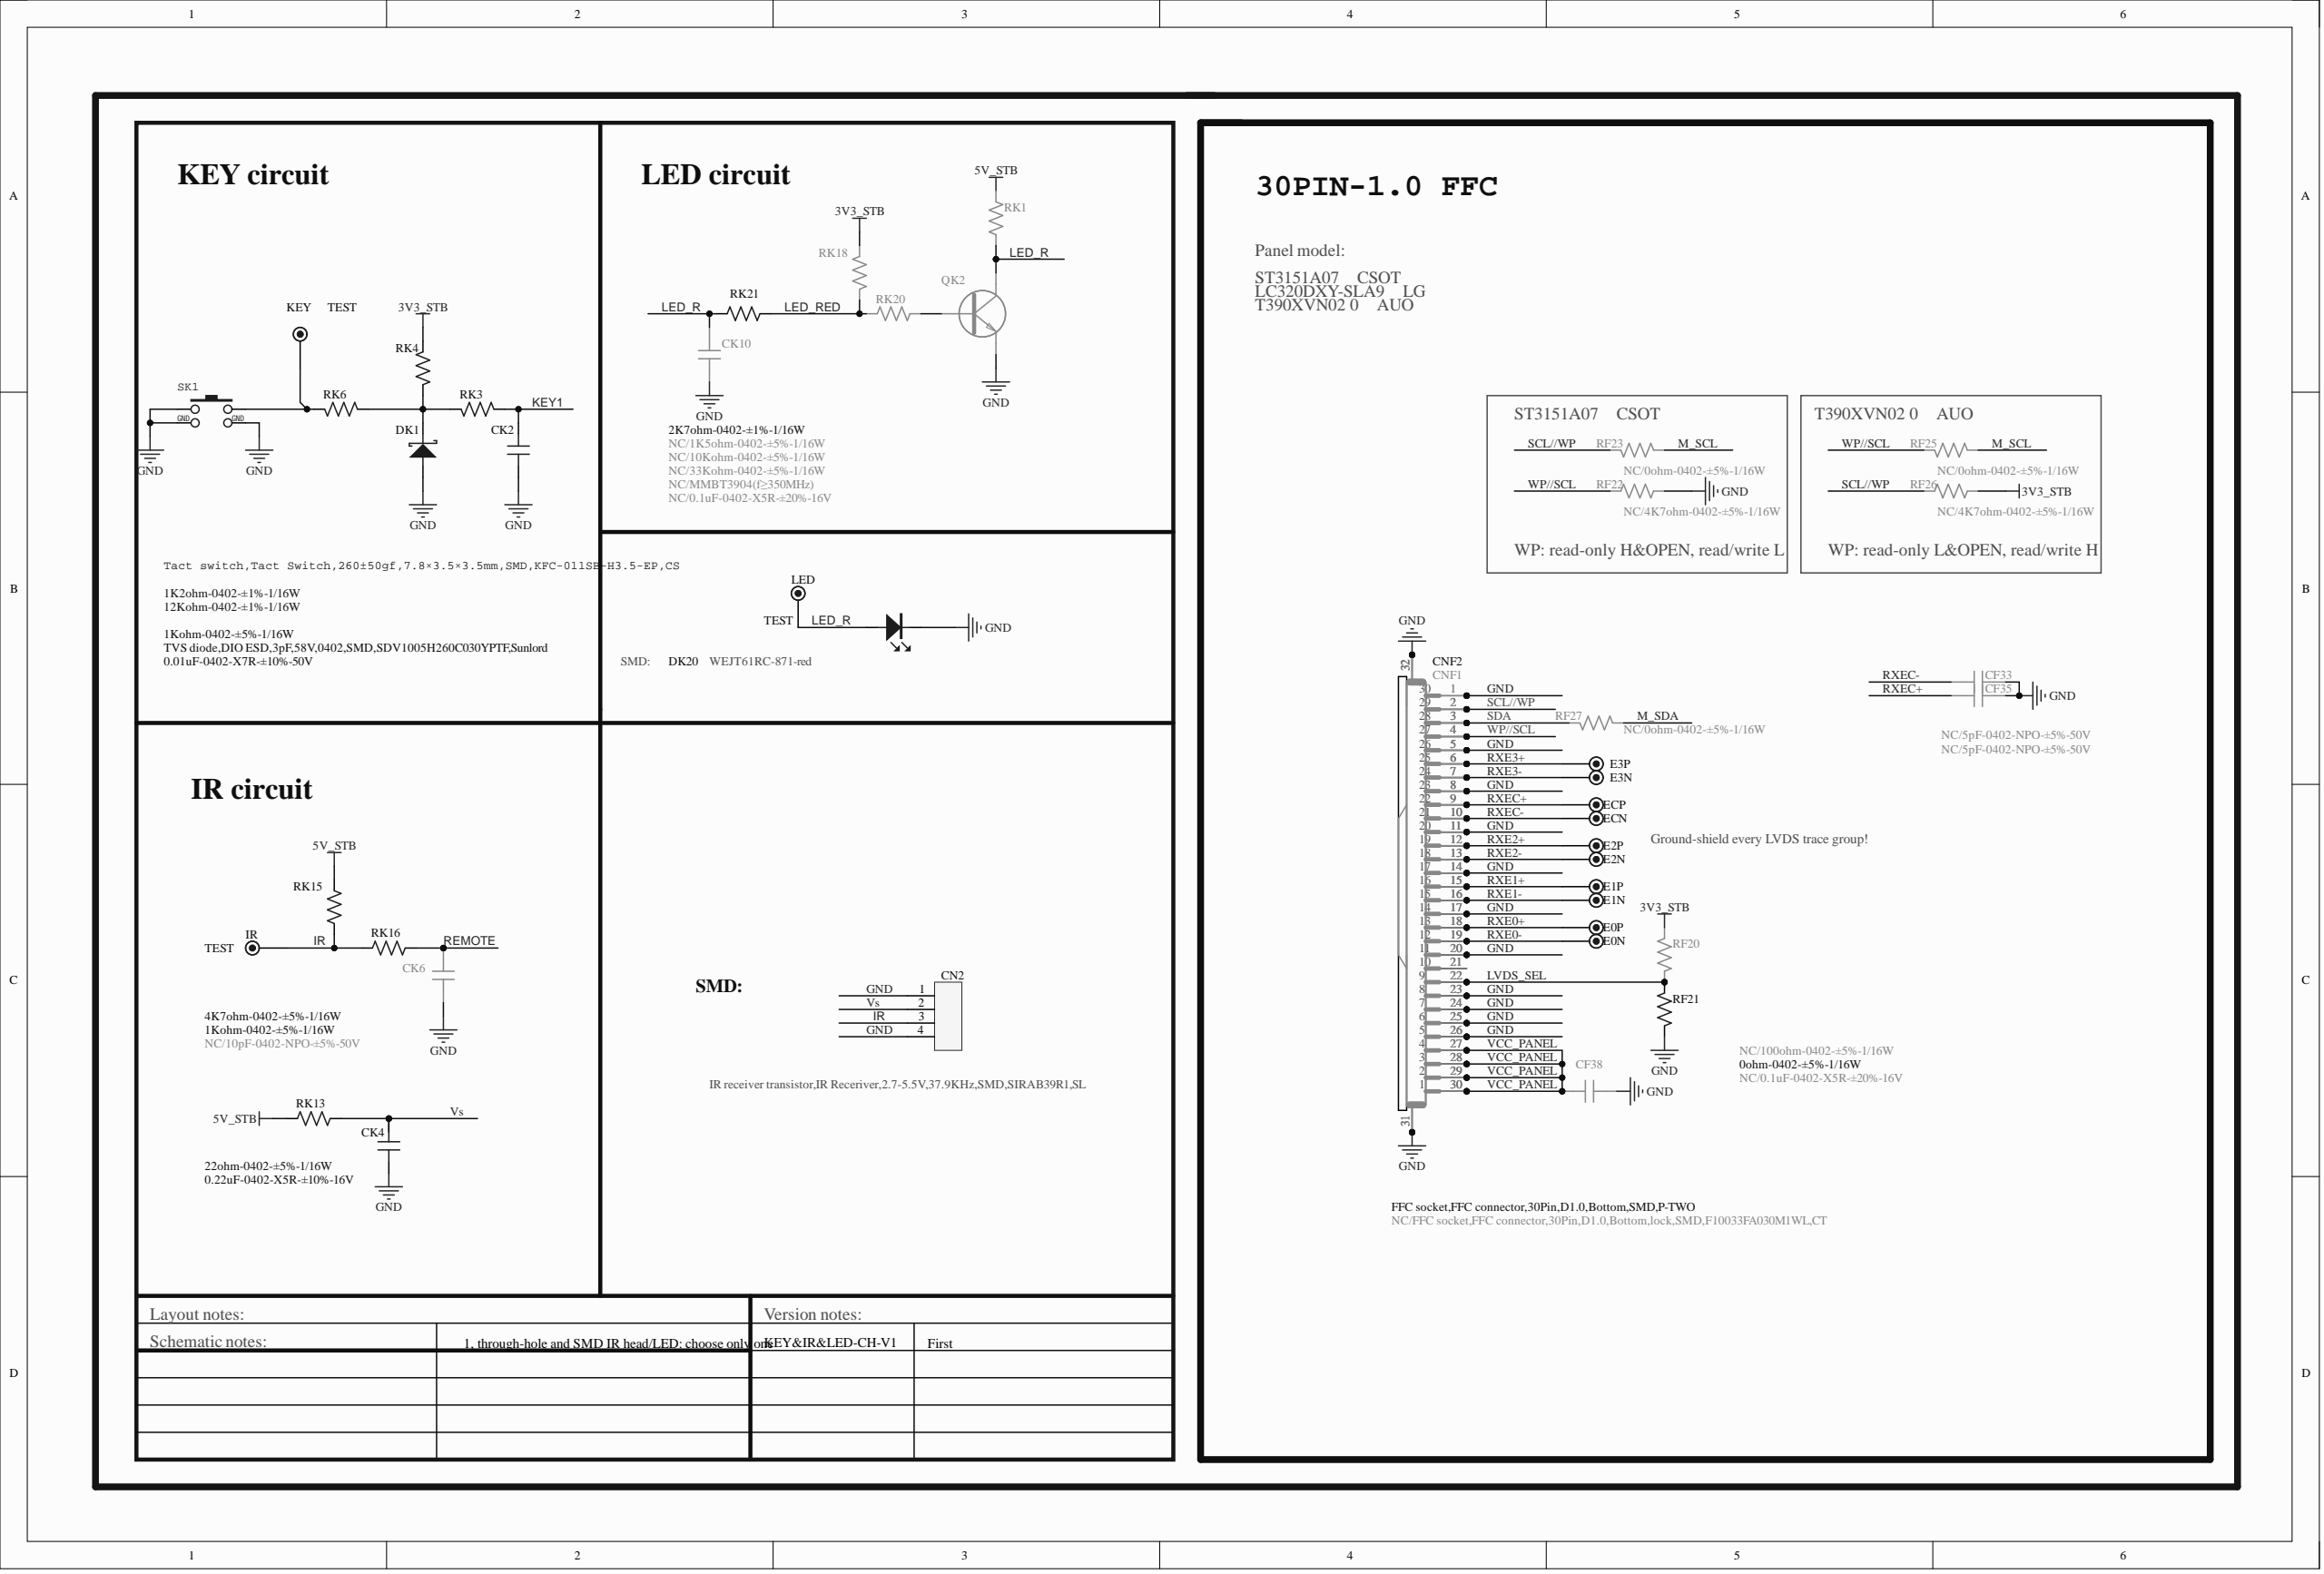Circuit board | Altium Designer | 574 parts | 274 nets | one sheet of the schematic
Parts on this sheet (reference | value | footprint):
CF33 | NC/5pF-0402-NPO-±5%-50V | C0402
CF35 | NC/5pF-0402-NPO-±5%-50V | C0402
CF38 | NC/0.1uF-0402-X5R-±20%-16V | C0402
CK2 | 0.01uF-0402-X7R-±10%-50V | C0402
CK4 | 0.22uF-0402-X5R-±10%-16V | C0402
CK6 | NC/10pF-0402-NPO-±5%-50V | C0402
CK10 | NC/0.1uF-0402-X5R-±20%-16V | C0402
CN2 | IR receiver transistor,IR Receriver,2.7-5.5V,37.9KHz,SMD,SIRAB39R1,SL | REMOTE-HS-1
CNF1 | NC/FFC socket,FFC connector,30Pin,D1.0,Bottom,lock,SMD,F10033FA030M1WL,CT | FFC30H/1.0S-7
CNF2 | FFC socket,FFC connector,30Pin,D1.0,Bottom,SMD,P-TWO | FFC30H/1.0S-1
DK1 | TVS diode,DIO ESD,3pF,58V,0402,SMD,SDV1005H260C030YPTF,Sunlord | DIODE-S0402
DK20 | WEJT61RC-871-red | DIODE-S0603
E0N | TEST | TP
E0P | TEST | TP
E1N | TEST | TP
E1P | TEST | TP
E2N | TEST | TP
E2P | TEST | TP
E3N | TEST | TP
E3P | TEST | TP
ECN | TEST | TP
ECP | TEST | TP
IR | TEST | TP
KEY | TEST | TP
LED | TEST | TP
QK2 | NC/MMBT3904(f=350MHz) | SOT-23
RF20 | NC/100ohm-0402-±5%-1/16W | R0402
RF21 | 0ohm-0402-±5%-1/16W | R0402
RF22 | NC/4K7ohm-0402-±5%-1/16W | R0402
RF23 | NC/0ohm-0402-±5%-1/16W | R0402
RF25 | NC/0ohm-0402-±5%-1/16W | R0402
RF26 | NC/4K7ohm-0402-±5%-1/16W | R0402
RF27 | NC/0ohm-0402-±5%-1/16W | R0402
RK1 | NC/1K5ohm-0402-±5%-1/16W | R0402
RK3 | 1Kohm-0402-±5%-1/16W | R0402
RK4 | 12Kohm-0402-±1%-1/16W | R0402
RK6 | 1K2ohm-0402-±1%-1/16W | R0402
RK13 | 22ohm-0402-±5%-1/16W | R0402
RK15 | 4K7ohm-0402-±5%-1/16W | R0402
RK16 | 1Kohm-0402-±5%-1/16W | R0402
RK18 | NC/33Kohm-0402-±5%-1/16W | R0402
RK20 | NC/10Kohm-0402-±5%-1/16W | R0402
RK21 | 2K7ohm-0402-±1%-1/16W | R0402
SK1 | Tact switch,Tact Switch,260±50gf,7.8×3.5×3.5mm,SMD,KFC-011SB-H3.5-EP,CS | KEY-HS-5
Nets of these parts (net: part-pin ...):
WP//SCL: RF22-2 RF25-2 CNF1-4 CNF2-4
Vs: CK4-1 CN2-2 RK13-2
VCC_PANEL: CF38-1 CNF1-27 CNF1-28 CNF1-29 CNF1-30 CNF2-27 CNF2-28 CNF2-29 CNF2-30
SDA: RF27-2 CNF1-3 CNF2-3
SCL//WP: RF23-2 RF26-2 CNF1-2 CNF2-2
RXEC-: CF33-2 ECN-1 CNF1-10 CNF2-10
RXEC+: CF35-2 ECP-1 CNF1-9 CNF2-9
RXE3-: E3N-1 CNF1-7 CNF2-7
RXE3+: E3P-1 CNF1-6 CNF2-6
RXE2-: E2N-1 CNF1-13 CNF2-13
RXE2+: E2P-1 CNF1-12 CNF2-12
RXE1-: E1N-1 CNF1-16 CNF2-16
RXE1+: E1P-1 CNF1-15 CNF2-15
RXE0-: E0N-1 CNF1-19 CNF2-19
RXE0+: E0P-1 CNF1-18 CNF2-18
REMOTE: CK6-2 RK16-1
NetQK2_B: QK2-B RK20-1
NetKEY_1: KEY-1 RK6-2 SK1-2
NetDK1_K: DK1-K RK3-2 RK4-1 RK6-1
M_SDA: RF27-1
M_SCL: RF23-1 RF25-1
LVDS_SEL: RF20-1 RF21-2 CNF1-22 CNF2-22
LED_RED: RK18-1 RK20-2 RK21-1
LED_R: CK10-2 DK20-A LED-1 QK2-C RK1-1 RK21-2
KEY1: CK2-1 RK3-1
IR: CN2-3 IR-1 RK15-2 RK16-2
GND: CF33-1 CF35-1 CF38-2 CK2-2 CK4-2 CK6-1 CK10-1 CN2-1 CN2-4 DK1-A DK20-K QK2-E RF21-1 RF22-1 SK1-1 SK1-3 SK1-4 CNF1-1 CNF1-5 CNF1-8 CNF1-11 CNF1-14 CNF1-17 CNF1-20 CNF1-23 CNF1-24 CNF1-25 CNF1-26 CNF1-31 CNF1-32 CNF2-1 CNF2-5 CNF2-8 CNF2-11 CNF2-14 CNF2-17 CNF2-20 CNF2-23 CNF2-24 CNF2-25 CNF2-26 CNF2-31 CNF2-32
5V_STB: RK1-2 RK13-1 RK15-1
3V3_STB: RF20-2 RF26-1 RK4-2 RK18-2